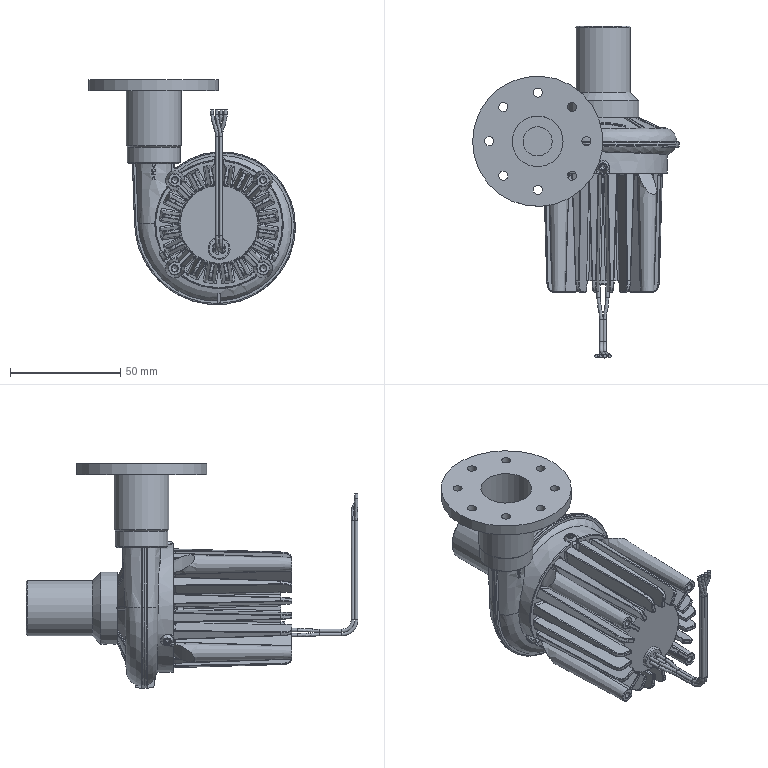Part | STEP file | u71hl-024km-41 | 1 solid | 1285 faces | box 93.697 x 150.3 x 101.919 mm | volume 187964 mm3 | spline 410 | plane 361 | cylinder 271 | cone 104 | torus 93 | sphere 46 | commonest cylinder face diameters 1.6 x60 0.6 x41 1 x32 1.5 x20 35.153 x20 0.8 x18